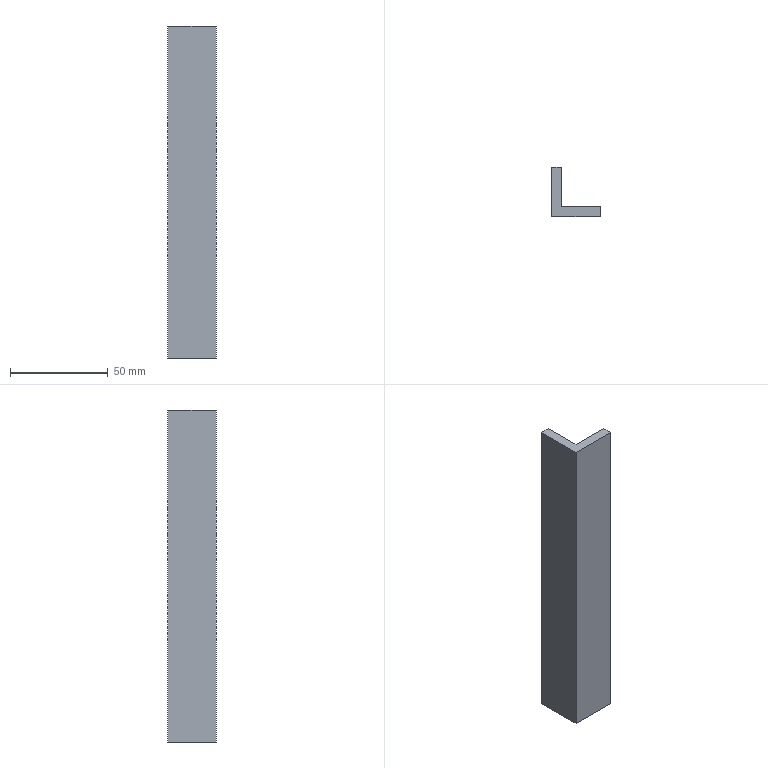Part | SolidWorks | features Extrusion 1 | 1 solid | 8 faces | box 25 x 25 x 170 mm | volume 38250 mm3 | plane 8
STEP:
#1=CARTESIAN_POINT('',(0.,0.,0.));
#2=VERTEX_POINT('',#1);
#3=CARTESIAN_POINT('',(25.,0.,0.));
#4=VERTEX_POINT('',#3);
#5=CARTESIAN_POINT('',(25.,0.,0.));
#6=DIRECTION('',(1.,0.,0.));
#7=VECTOR('',#6,1000.);
#8=LINE('',#5,#7);
#9=EDGE_CURVE('',#2,#4,#8,.T.);
#10=ORIENTED_EDGE('',*,*,#9,.T.);
#11=CARTESIAN_POINT('',(25.,0.,170.));
#12=VERTEX_POINT('',#11);
#13=CARTESIAN_POINT('',(25.,0.,170.));
#14=DIRECTION('',(0.,0.,-1.));
#15=VECTOR('',#14,1000.);
#16=LINE('',#13,#15);
#17=EDGE_CURVE('',#12,#4,#16,.T.);
#18=ORIENTED_EDGE('',*,*,#17,.F.);
#19=CARTESIAN_POINT('',(0.,0.,170.));
#20=VERTEX_POINT('',#19);
#21=CARTESIAN_POINT('',(25.,0.,170.));
#22=DIRECTION('',(1.,0.,0.));
#23=VECTOR('',#22,1000.);
#24=LINE('',#21,#23);
#25=EDGE_CURVE('',#20,#12,#24,.T.);
#26=ORIENTED_EDGE('',*,*,#25,.F.);
#27=CARTESIAN_POINT('',(0.,0.,170.));
#28=DIRECTION('',(0.,0.,-1.));
#29=VECTOR('',#28,1000.);
#30=LINE('',#27,#29);
#31=EDGE_CURVE('',#20,#2,#30,.T.);
#32=ORIENTED_EDGE('',*,*,#31,.T.);
#33=EDGE_LOOP('',(#10,#18,#26,#32));
#34=FACE_OUTER_BOUND('',#33,.T.);
#35=CARTESIAN_POINT('',(25.,0.,170.));
#36=DIRECTION('',(0.,1.,0.));
#37=DIRECTION('',(-1.,0.,0.));
#38=AXIS2_PLACEMENT_3D('',#35,#36,#37);
#39=PLANE('',#38);
#40=ADVANCED_FACE('',(#34),#39,.F.);
#41=CARTESIAN_POINT('',(25.,5.,0.));
#42=VERTEX_POINT('',#41);
#43=CARTESIAN_POINT('',(25.,5.,0.));
#44=DIRECTION('',(0.,1.,0.));
#45=VECTOR('',#44,1000.);
#46=LINE('',#43,#45);
#47=EDGE_CURVE('',#4,#42,#46,.T.);
#48=ORIENTED_EDGE('',*,*,#47,.T.);
#49=CARTESIAN_POINT('',(25.,5.,170.));
#50=VERTEX_POINT('',#49);
#51=CARTESIAN_POINT('',(25.,5.,170.));
#52=DIRECTION('',(0.,0.,-1.));
#53=VECTOR('',#52,1000.);
#54=LINE('',#51,#53);
#55=EDGE_CURVE('',#50,#42,#54,.T.);
#56=ORIENTED_EDGE('',*,*,#55,.F.);
#57=CARTESIAN_POINT('',(25.,5.,170.));
#58=DIRECTION('',(0.,1.,0.));
#59=VECTOR('',#58,1000.);
#60=LINE('',#57,#59);
#61=EDGE_CURVE('',#12,#50,#60,.T.);
#62=ORIENTED_EDGE('',*,*,#61,.F.);
#63=ORIENTED_EDGE('',*,*,#17,.T.);
#64=EDGE_LOOP('',(#48,#56,#62,#63));
#65=FACE_OUTER_BOUND('',#64,.T.);
#66=CARTESIAN_POINT('',(25.,5.,170.));
#67=DIRECTION('',(-1.,0.,0.));
#68=DIRECTION('',(0.,0.,1.));
#69=AXIS2_PLACEMENT_3D('',#66,#67,#68);
#70=PLANE('',#69);
#71=ADVANCED_FACE('',(#65),#70,.F.);
#72=CARTESIAN_POINT('',(5.,5.,0.));
#73=VERTEX_POINT('',#72);
#74=CARTESIAN_POINT('',(5.,5.,0.));
#75=DIRECTION('',(-1.,0.,0.));
#76=VECTOR('',#75,1000.);
#77=LINE('',#74,#76);
#78=EDGE_CURVE('',#42,#73,#77,.T.);
#79=ORIENTED_EDGE('',*,*,#78,.T.);
#80=CARTESIAN_POINT('',(5.,5.,170.));
#81=VERTEX_POINT('',#80);
#82=CARTESIAN_POINT('',(5.,5.,170.));
#83=DIRECTION('',(0.,0.,-1.));
#84=VECTOR('',#83,1000.);
#85=LINE('',#82,#84);
#86=EDGE_CURVE('',#81,#73,#85,.T.);
#87=ORIENTED_EDGE('',*,*,#86,.F.);
#88=CARTESIAN_POINT('',(5.,5.,170.));
#89=DIRECTION('',(-1.,0.,0.));
#90=VECTOR('',#89,1000.);
#91=LINE('',#88,#90);
#92=EDGE_CURVE('',#50,#81,#91,.T.);
#93=ORIENTED_EDGE('',*,*,#92,.F.);
#94=ORIENTED_EDGE('',*,*,#55,.T.);
#95=EDGE_LOOP('',(#79,#87,#93,#94));
#96=FACE_OUTER_BOUND('',#95,.T.);
#97=CARTESIAN_POINT('',(5.,5.,170.));
#98=DIRECTION('',(0.,-1.,0.));
#99=DIRECTION('',(0.,0.,-1.));
#100=AXIS2_PLACEMENT_3D('',#97,#98,#99);
#101=PLANE('',#100);
#102=ADVANCED_FACE('',(#96),#101,.F.);
#103=CARTESIAN_POINT('',(5.,25.,0.));
#104=VERTEX_POINT('',#103);
#105=CARTESIAN_POINT('',(5.,25.,0.));
#106=DIRECTION('',(0.,1.,0.));
#107=VECTOR('',#106,1000.);
#108=LINE('',#105,#107);
#109=EDGE_CURVE('',#73,#104,#108,.T.);
#110=ORIENTED_EDGE('',*,*,#109,.T.);
#111=CARTESIAN_POINT('',(5.,25.,170.));
#112=VERTEX_POINT('',#111);
#113=CARTESIAN_POINT('',(5.,25.,170.));
#114=DIRECTION('',(0.,0.,-1.));
#115=VECTOR('',#114,1000.);
#116=LINE('',#113,#115);
#117=EDGE_CURVE('',#112,#104,#116,.T.);
#118=ORIENTED_EDGE('',*,*,#117,.F.);
#119=CARTESIAN_POINT('',(5.,25.,170.));
#120=DIRECTION('',(0.,1.,0.));
#121=VECTOR('',#120,1000.);
#122=LINE('',#119,#121);
#123=EDGE_CURVE('',#81,#112,#122,.T.);
#124=ORIENTED_EDGE('',*,*,#123,.F.);
#125=ORIENTED_EDGE('',*,*,#86,.T.);
#126=EDGE_LOOP('',(#110,#118,#124,#125));
#127=FACE_OUTER_BOUND('',#126,.T.);
#128=CARTESIAN_POINT('',(5.,25.,170.));
#129=DIRECTION('',(-1.,0.,0.));
#130=DIRECTION('',(0.,-1.,0.));
#131=AXIS2_PLACEMENT_3D('',#128,#129,#130);
#132=PLANE('',#131);
#133=ADVANCED_FACE('',(#127),#132,.F.);
#134=CARTESIAN_POINT('',(0.,25.,0.));
#135=VERTEX_POINT('',#134);
#136=CARTESIAN_POINT('',(0.,25.,0.));
#137=DIRECTION('',(-1.,0.,0.));
#138=VECTOR('',#137,1000.);
#139=LINE('',#136,#138);
#140=EDGE_CURVE('',#104,#135,#139,.T.);
#141=ORIENTED_EDGE('',*,*,#140,.T.);
#142=CARTESIAN_POINT('',(0.,25.,170.));
#143=VERTEX_POINT('',#142);
#144=CARTESIAN_POINT('',(0.,25.,170.));
#145=DIRECTION('',(0.,0.,-1.));
#146=VECTOR('',#145,1000.);
#147=LINE('',#144,#146);
#148=EDGE_CURVE('',#143,#135,#147,.T.);
#149=ORIENTED_EDGE('',*,*,#148,.F.);
#150=CARTESIAN_POINT('',(0.,25.,170.));
#151=DIRECTION('',(-1.,0.,0.));
#152=VECTOR('',#151,1000.);
#153=LINE('',#150,#152);
#154=EDGE_CURVE('',#112,#143,#153,.T.);
#155=ORIENTED_EDGE('',*,*,#154,.F.);
#156=ORIENTED_EDGE('',*,*,#117,.T.);
#157=EDGE_LOOP('',(#141,#149,#155,#156));
#158=FACE_OUTER_BOUND('',#157,.T.);
#159=CARTESIAN_POINT('',(0.,25.,170.));
#160=DIRECTION('',(0.,-1.,0.));
#161=DIRECTION('',(0.,0.,-1.));
#162=AXIS2_PLACEMENT_3D('',#159,#160,#161);
#163=PLANE('',#162);
#164=ADVANCED_FACE('',(#158),#163,.F.);
#165=CARTESIAN_POINT('',(0.,0.,0.));
#166=DIRECTION('',(0.,-1.,0.));
#167=VECTOR('',#166,1000.);
#168=LINE('',#165,#167);
#169=EDGE_CURVE('',#135,#2,#168,.T.);
#170=ORIENTED_EDGE('',*,*,#169,.T.);
#171=ORIENTED_EDGE('',*,*,#31,.F.);
#172=CARTESIAN_POINT('',(0.,0.,170.));
#173=DIRECTION('',(0.,-1.,0.));
#174=VECTOR('',#173,1000.);
#175=LINE('',#172,#174);
#176=EDGE_CURVE('',#143,#20,#175,.T.);
#177=ORIENTED_EDGE('',*,*,#176,.F.);
#178=ORIENTED_EDGE('',*,*,#148,.T.);
#179=EDGE_LOOP('',(#170,#171,#177,#178));
#180=FACE_OUTER_BOUND('',#179,.T.);
#181=CARTESIAN_POINT('',(0.,0.,170.));
#182=DIRECTION('',(1.,0.,0.));
#183=DIRECTION('',(0.,1.,0.));
#184=AXIS2_PLACEMENT_3D('',#181,#182,#183);
#185=PLANE('',#184);
#186=ADVANCED_FACE('',(#180),#185,.F.);
#187=ORIENTED_EDGE('',*,*,#25,.T.);
#188=ORIENTED_EDGE('',*,*,#61,.T.);
#189=ORIENTED_EDGE('',*,*,#92,.T.);
#190=ORIENTED_EDGE('',*,*,#123,.T.);
#191=ORIENTED_EDGE('',*,*,#154,.T.);
#192=ORIENTED_EDGE('',*,*,#176,.T.);
#193=EDGE_LOOP('',(#187,#188,#189,#190,#191,#192));
#194=FACE_OUTER_BOUND('',#193,.T.);
#195=CARTESIAN_POINT('',(0.,0.,170.));
#196=DIRECTION('',(0.,0.,-1.));
#197=DIRECTION('',(-1.,0.,0.));
#198=AXIS2_PLACEMENT_3D('',#195,#196,#197);
#199=PLANE('',#198);
#200=ADVANCED_FACE('',(#194),#199,.F.);
#201=ORIENTED_EDGE('',*,*,#9,.F.);
#202=ORIENTED_EDGE('',*,*,#169,.F.);
#203=ORIENTED_EDGE('',*,*,#140,.F.);
#204=ORIENTED_EDGE('',*,*,#109,.F.);
#205=ORIENTED_EDGE('',*,*,#78,.F.);
#206=ORIENTED_EDGE('',*,*,#47,.F.);
#207=EDGE_LOOP('',(#201,#202,#203,#204,#205,#206));
#208=FACE_OUTER_BOUND('',#207,.T.);
#209=CARTESIAN_POINT('',(0.,0.,0.));
#210=DIRECTION('',(0.,0.,-1.));
#211=DIRECTION('',(-1.,0.,0.));
#212=AXIS2_PLACEMENT_3D('',#209,#210,#211);
#213=PLANE('',#212);
#214=ADVANCED_FACE('',(#208),#213,.T.);
#215=CLOSED_SHELL('',(#40,#71,#102,#133,#164,#186,#200,#214));
#216=MANIFOLD_SOLID_BREP('',#215);
#217=CARTESIAN_POINT('',(0.,0.,0.));
#218=DIRECTION('',(0.,0.,1.));
#219=DIRECTION('',(1.,0.,0.));
#220=AXIS2_PLACEMENT_3D('',#217,#218,#219);
#221=(LENGTH_UNIT()NAMED_UNIT(*)SI_UNIT(.MILLI.,.METRE.));
#222=UNCERTAINTY_MEASURE_WITH_UNIT(LENGTH_MEASURE(0.00001),#221,'','');
#223=(NAMED_UNIT(*)PLANE_ANGLE_UNIT()SI_UNIT($,.RADIAN.));
#224=(NAMED_UNIT(*)SI_UNIT($,.STERADIAN.)SOLID_ANGLE_UNIT());
#225=(GEOMETRIC_REPRESENTATION_CONTEXT(3)GLOBAL_UNCERTAINTY_ASSIGNED_CONTEXT((#222))GLOBAL_UNIT_ASSIGNED_CONTEXT((#221,#223,#224))REPRESENTATION_CONTEXT('',''));
#226=ADVANCED_BREP_SHAPE_REPRESENTATION('',(#216,#220),#225);